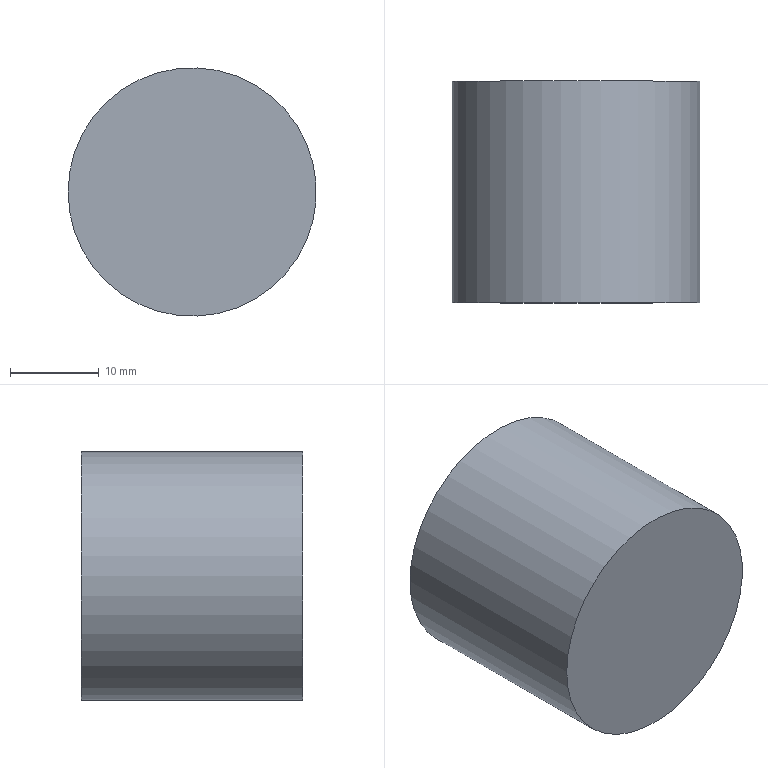Part | NX | features solid 2 | 1 solid | 3 faces | box 28 x 25 x 28 mm | volume 15394 mm3 | plane 2 | cylinder 1 | commonest cylinder face diameters 28 x1
STEP:
#1=CARTESIAN_POINT('',(586.,-710.,-395.));
#2=VERTEX_POINT('',#1);
#3=CARTESIAN_POINT('',(600.,-710.,-395.));
#4=DIRECTION('',(0.,1.,0.));
#5=DIRECTION('',(-1.,0.,0.));
#6=AXIS2_PLACEMENT_3D('',#3,#4,#5);
#7=CIRCLE('',#6,14.);
#8=EDGE_CURVE('',#2,#2,#7,.T.);
#9=ORIENTED_EDGE('',*,*,#8,.F.);
#10=EDGE_LOOP('',(#9));
#11=FACE_BOUND('',#10,.T.);
#12=CARTESIAN_POINT('',(586.,-735.,-395.));
#13=VERTEX_POINT('',#12);
#14=CARTESIAN_POINT('',(600.,-735.,-395.));
#15=DIRECTION('',(0.,1.,0.));
#16=DIRECTION('',(-1.,0.,0.));
#17=AXIS2_PLACEMENT_3D('',#14,#15,#16);
#18=CIRCLE('',#17,14.);
#19=EDGE_CURVE('',#13,#13,#18,.T.);
#20=ORIENTED_EDGE('',*,*,#19,.T.);
#21=EDGE_LOOP('',(#20));
#22=FACE_BOUND('',#21,.T.);
#23=CARTESIAN_POINT('',(600.,-710.,-395.));
#24=DIRECTION('',(0.,-1.,0.));
#25=DIRECTION('',(0.,0.,-1.));
#26=AXIS2_PLACEMENT_3D('',#23,#24,#25);
#27=CYLINDRICAL_SURFACE('',#26,14.);
#28=ADVANCED_FACE('',(#11,#22),#27,.T.);
#29=ORIENTED_EDGE('',*,*,#8,.T.);
#30=EDGE_LOOP('',(#29));
#31=FACE_BOUND('',#30,.T.);
#32=CARTESIAN_POINT('',(600.,-710.,-395.));
#33=DIRECTION('',(0.,1.,0.));
#34=DIRECTION('',(-1.,0.,0.));
#35=AXIS2_PLACEMENT_3D('',#32,#33,#34);
#36=PLANE('',#35);
#37=ADVANCED_FACE('',(#31),#36,.T.);
#38=ORIENTED_EDGE('',*,*,#19,.F.);
#39=EDGE_LOOP('',(#38));
#40=FACE_BOUND('',#39,.T.);
#41=CARTESIAN_POINT('',(600.,-735.,-395.));
#42=DIRECTION('',(0.,1.,0.));
#43=DIRECTION('',(-1.,0.,0.));
#44=AXIS2_PLACEMENT_3D('',#41,#42,#43);
#45=PLANE('',#44);
#46=ADVANCED_FACE('',(#40),#45,.F.);
#47=CLOSED_SHELL('',(#28,#37,#46));
#48=MANIFOLD_SOLID_BREP('',#47);
#49=(LENGTH_UNIT()NAMED_UNIT(*)SI_UNIT(.MILLI.,.METRE.));
#50=UNCERTAINTY_MEASURE_WITH_UNIT(LENGTH_MEASURE(0.00001),#49,'','');
#51=(NAMED_UNIT(*)PLANE_ANGLE_UNIT()SI_UNIT($,.RADIAN.));
#52=(NAMED_UNIT(*)SI_UNIT($,.STERADIAN.)SOLID_ANGLE_UNIT());
#53=(GEOMETRIC_REPRESENTATION_CONTEXT(3)GLOBAL_UNCERTAINTY_ASSIGNED_CONTEXT((#50))GLOBAL_UNIT_ASSIGNED_CONTEXT((#49,#51,#52))REPRESENTATION_CONTEXT('',''));
#54=ADVANCED_BREP_SHAPE_REPRESENTATION('',(#48),#53);